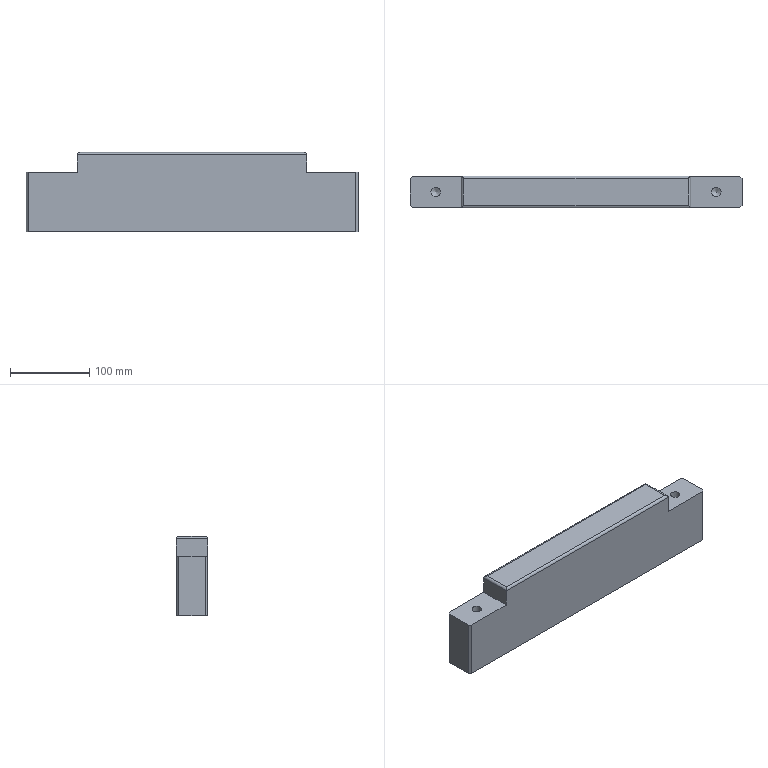Part | NX | features solid 2 | 1 solid | 26 faces | box 420 x 40 x 100 mm | volume 1534744 mm3 | plane 16 | cylinder 8 | cone 2 | commonest cylinder face diameters 6 x4 9 x2 12 x2
STEP:
#1=CARTESIAN_POINT('',(-323.,-106.5,359.));
#2=VERTEX_POINT('',#1);
#3=CARTESIAN_POINT('',(-323.,-106.5,363.5));
#4=DIRECTION('',(0.,-1.,0.));
#5=DIRECTION('',(0.,0.,-1.));
#6=AXIS2_PLACEMENT_3D('',#3,#4,#5);
#7=CIRCLE('',#6,4.5);
#8=EDGE_CURVE('',#2,#2,#7,.T.);
#9=ORIENTED_EDGE('',*,*,#8,.T.);
#10=EDGE_LOOP('',(#9));
#11=FACE_BOUND('',#10,.T.);
#12=CARTESIAN_POINT('',(-268.,-106.5,359.));
#13=VERTEX_POINT('',#12);
#14=CARTESIAN_POINT('',(-268.,-106.5,363.5));
#15=DIRECTION('',(0.,-1.,0.));
#16=DIRECTION('',(0.,0.,-1.));
#17=AXIS2_PLACEMENT_3D('',#14,#15,#16);
#18=CIRCLE('',#17,4.5);
#19=EDGE_CURVE('',#13,#13,#18,.T.);
#20=ORIENTED_EDGE('',*,*,#19,.T.);
#21=EDGE_LOOP('',(#20));
#22=FACE_BOUND('',#21,.T.);
#23=CARTESIAN_POINT('',(-150.,-106.5,402.));
#24=VERTEX_POINT('',#23);
#25=CARTESIAN_POINT('',(-440.,-106.5,402.));
#26=VERTEX_POINT('',#25);
#27=CARTESIAN_POINT('',(-440.,-106.5,402.));
#28=DIRECTION('',(-1.,0.,0.));
#29=VECTOR('',#28,1000.);
#30=LINE('',#27,#29);
#31=EDGE_CURVE('',#24,#26,#30,.T.);
#32=ORIENTED_EDGE('',*,*,#31,.F.);
#33=CARTESIAN_POINT('',(-150.,-106.5,380.));
#34=VERTEX_POINT('',#33);
#35=CARTESIAN_POINT('',(-150.,-106.5,380.));
#36=DIRECTION('',(0.,0.,1.));
#37=VECTOR('',#36,1000.);
#38=LINE('',#35,#37);
#39=EDGE_CURVE('',#34,#24,#38,.T.);
#40=ORIENTED_EDGE('',*,*,#39,.F.);
#41=CARTESIAN_POINT('',(-88.,-106.5,380.));
#42=VERTEX_POINT('',#41);
#43=CARTESIAN_POINT('',(-500.,-106.5,380.));
#44=DIRECTION('',(1.,0.,0.));
#45=VECTOR('',#44,1000.);
#46=LINE('',#43,#45);
#47=EDGE_CURVE('',#34,#42,#46,.T.);
#48=ORIENTED_EDGE('',*,*,#47,.T.);
#49=CARTESIAN_POINT('',(-88.,-106.5,305.));
#50=VERTEX_POINT('',#49);
#51=CARTESIAN_POINT('',(-88.,-106.5,380.));
#52=DIRECTION('',(0.,0.,1.));
#53=VECTOR('',#52,1000.);
#54=LINE('',#51,#53);
#55=EDGE_CURVE('',#50,#42,#54,.T.);
#56=ORIENTED_EDGE('',*,*,#55,.F.);
#57=CARTESIAN_POINT('',(-502.,-106.5,305.));
#58=VERTEX_POINT('',#57);
#59=CARTESIAN_POINT('',(-570.,-106.5,305.));
#60=DIRECTION('',(1.,0.,0.));
#61=VECTOR('',#60,1000.);
#62=LINE('',#59,#61);
#63=EDGE_CURVE('',#58,#50,#62,.T.);
#64=ORIENTED_EDGE('',*,*,#63,.F.);
#65=CARTESIAN_POINT('',(-502.,-106.5,380.));
#66=VERTEX_POINT('',#65);
#67=CARTESIAN_POINT('',(-502.,-106.5,380.));
#68=DIRECTION('',(0.,0.,-1.));
#69=VECTOR('',#68,1000.);
#70=LINE('',#67,#69);
#71=EDGE_CURVE('',#66,#58,#70,.T.);
#72=ORIENTED_EDGE('',*,*,#71,.F.);
#73=CARTESIAN_POINT('',(-440.,-106.5,380.));
#74=VERTEX_POINT('',#73);
#75=CARTESIAN_POINT('',(-570.,-106.5,380.));
#76=DIRECTION('',(1.,0.,0.));
#77=VECTOR('',#76,1000.);
#78=LINE('',#75,#77);
#79=EDGE_CURVE('',#66,#74,#78,.T.);
#80=ORIENTED_EDGE('',*,*,#79,.T.);
#81=CARTESIAN_POINT('',(-440.,-106.5,405.));
#82=DIRECTION('',(0.,0.,-1.));
#83=VECTOR('',#82,1000.);
#84=LINE('',#81,#83);
#85=EDGE_CURVE('',#74,#26,#84,.F.);
#86=ORIENTED_EDGE('',*,*,#85,.T.);
#87=EDGE_LOOP('',(#32,#40,#48,#56,#64,#72,#80,#86));
#88=FACE_BOUND('',#87,.T.);
#89=CARTESIAN_POINT('',(-570.,-106.5,380.));
#90=DIRECTION('',(0.,-1.,0.));
#91=DIRECTION('',(0.,0.,1.));
#92=AXIS2_PLACEMENT_3D('',#89,#90,#91);
#93=PLANE('',#92);
#94=ADVANCED_FACE('',(#11,#22,#88),#93,.F.);
#95=ORIENTED_EDGE('',*,*,#63,.T.);
#96=CARTESIAN_POINT('',(-85.,-109.5,305.));
#97=VERTEX_POINT('',#96);
#98=CARTESIAN_POINT('',(-85.,-109.5,305.));
#99=DIRECTION('',(0.7071,-0.7071,0.));
#100=VECTOR('',#99,1000.);
#101=LINE('',#98,#100);
#102=EDGE_CURVE('',#97,#50,#101,.F.);
#103=ORIENTED_EDGE('',*,*,#102,.F.);
#104=CARTESIAN_POINT('',(-85.,-143.5,305.));
#105=VERTEX_POINT('',#104);
#106=CARTESIAN_POINT('',(-85.,-106.5,305.));
#107=DIRECTION('',(0.,-1.,0.));
#108=VECTOR('',#107,1000.);
#109=LINE('',#106,#108);
#110=EDGE_CURVE('',#97,#105,#109,.T.);
#111=ORIENTED_EDGE('',*,*,#110,.T.);
#112=CARTESIAN_POINT('',(-88.,-146.5,305.));
#113=VERTEX_POINT('',#112);
#114=CARTESIAN_POINT('',(-88.,-146.5,305.));
#115=DIRECTION('',(-0.7071,-0.7071,0.));
#116=VECTOR('',#115,1000.);
#117=LINE('',#114,#116);
#118=EDGE_CURVE('',#113,#105,#117,.F.);
#119=ORIENTED_EDGE('',*,*,#118,.F.);
#120=CARTESIAN_POINT('',(-502.,-146.5,305.));
#121=VERTEX_POINT('',#120);
#122=CARTESIAN_POINT('',(-150.,-146.5,305.));
#123=DIRECTION('',(-1.,0.,0.));
#124=VECTOR('',#123,1000.);
#125=LINE('',#122,#124);
#126=EDGE_CURVE('',#113,#121,#125,.T.);
#127=ORIENTED_EDGE('',*,*,#126,.T.);
#128=CARTESIAN_POINT('',(-505.,-143.5,305.));
#129=VERTEX_POINT('',#128);
#130=CARTESIAN_POINT('',(-505.,-143.5,305.));
#131=DIRECTION('',(-0.7071,0.7071,0.));
#132=VECTOR('',#131,1000.);
#133=LINE('',#130,#132);
#134=EDGE_CURVE('',#129,#121,#133,.F.);
#135=ORIENTED_EDGE('',*,*,#134,.F.);
#136=CARTESIAN_POINT('',(-505.,-109.5,305.));
#137=VERTEX_POINT('',#136);
#138=CARTESIAN_POINT('',(-505.,-137.5,305.));
#139=DIRECTION('',(0.,1.,0.));
#140=VECTOR('',#139,1000.);
#141=LINE('',#138,#140);
#142=EDGE_CURVE('',#129,#137,#141,.T.);
#143=ORIENTED_EDGE('',*,*,#142,.T.);
#144=CARTESIAN_POINT('',(-502.,-106.5,305.));
#145=DIRECTION('',(0.7071,0.7071,0.));
#146=VECTOR('',#145,1000.);
#147=LINE('',#144,#146);
#148=EDGE_CURVE('',#58,#137,#147,.F.);
#149=ORIENTED_EDGE('',*,*,#148,.F.);
#150=EDGE_LOOP('',(#95,#103,#111,#119,#127,#135,#143,#149));
#151=FACE_BOUND('',#150,.T.);
#152=CARTESIAN_POINT('',(-470.,-127.5,305.));
#153=DIRECTION('',(0.,0.,1.));
#154=DIRECTION('',(1.,0.,0.));
#155=AXIS2_PLACEMENT_3D('',#152,#153,#154);
#156=PLANE('',#155);
#157=ADVANCED_FACE('',(#151),#156,.F.);
#158=ORIENTED_EDGE('',*,*,#126,.F.);
#159=CARTESIAN_POINT('',(-88.,-146.5,380.));
#160=VERTEX_POINT('',#159);
#161=CARTESIAN_POINT('',(-88.,-146.5,380.));
#162=DIRECTION('',(0.,0.,-1.));
#163=VECTOR('',#162,1000.);
#164=LINE('',#161,#163);
#165=EDGE_CURVE('',#160,#113,#164,.T.);
#166=ORIENTED_EDGE('',*,*,#165,.F.);
#167=CARTESIAN_POINT('',(-150.,-146.5,380.));
#168=VERTEX_POINT('',#167);
#169=CARTESIAN_POINT('',(-80.,-146.5,380.));
#170=DIRECTION('',(-1.,0.,0.));
#171=VECTOR('',#170,1000.);
#172=LINE('',#169,#171);
#173=EDGE_CURVE('',#160,#168,#172,.T.);
#174=ORIENTED_EDGE('',*,*,#173,.T.);
#175=CARTESIAN_POINT('',(-150.,-146.5,402.));
#176=VERTEX_POINT('',#175);
#177=CARTESIAN_POINT('',(-150.,-146.5,405.));
#178=DIRECTION('',(0.,0.,1.));
#179=VECTOR('',#178,1000.);
#180=LINE('',#177,#179);
#181=EDGE_CURVE('',#168,#176,#180,.T.);
#182=ORIENTED_EDGE('',*,*,#181,.T.);
#183=CARTESIAN_POINT('',(-440.,-146.5,402.));
#184=VERTEX_POINT('',#183);
#185=CARTESIAN_POINT('',(-220.,-146.5,402.));
#186=DIRECTION('',(1.,0.,0.));
#187=VECTOR('',#186,1000.);
#188=LINE('',#185,#187);
#189=EDGE_CURVE('',#184,#176,#188,.T.);
#190=ORIENTED_EDGE('',*,*,#189,.F.);
#191=CARTESIAN_POINT('',(-440.,-146.5,380.));
#192=VERTEX_POINT('',#191);
#193=CARTESIAN_POINT('',(-440.,-146.5,380.));
#194=DIRECTION('',(0.,0.,-1.));
#195=VECTOR('',#194,1000.);
#196=LINE('',#193,#195);
#197=EDGE_CURVE('',#192,#184,#196,.F.);
#198=ORIENTED_EDGE('',*,*,#197,.F.);
#199=CARTESIAN_POINT('',(-502.,-146.5,380.));
#200=VERTEX_POINT('',#199);
#201=CARTESIAN_POINT('',(-150.,-146.5,380.));
#202=DIRECTION('',(-1.,0.,0.));
#203=VECTOR('',#202,1000.);
#204=LINE('',#201,#203);
#205=EDGE_CURVE('',#192,#200,#204,.T.);
#206=ORIENTED_EDGE('',*,*,#205,.T.);
#207=CARTESIAN_POINT('',(-502.,-146.5,380.));
#208=DIRECTION('',(0.,0.,1.));
#209=VECTOR('',#208,1000.);
#210=LINE('',#207,#209);
#211=EDGE_CURVE('',#121,#200,#210,.T.);
#212=ORIENTED_EDGE('',*,*,#211,.F.);
#213=EDGE_LOOP('',(#158,#166,#174,#182,#190,#198,#206,#212));
#214=FACE_BOUND('',#213,.T.);
#215=CARTESIAN_POINT('',(-150.,-146.5,380.));
#216=DIRECTION('',(0.,1.,0.));
#217=DIRECTION('',(0.,0.,-1.));
#218=AXIS2_PLACEMENT_3D('',#215,#216,#217);
#219=PLANE('',#218);
#220=ADVANCED_FACE('',(#214),#219,.F.);
#221=CARTESIAN_POINT('',(-153.,-143.5,405.));
#222=VERTEX_POINT('',#221);
#223=CARTESIAN_POINT('',(-437.,-143.5,405.));
#224=VERTEX_POINT('',#223);
#225=CARTESIAN_POINT('',(-440.,-143.5,405.));
#226=DIRECTION('',(1.,0.,0.));
#227=VECTOR('',#226,1000.);
#228=LINE('',#225,#227);
#229=EDGE_CURVE('',#222,#224,#228,.F.);
#230=ORIENTED_EDGE('',*,*,#229,.F.);
#231=CARTESIAN_POINT('',(-153.,-109.5,405.));
#232=VERTEX_POINT('',#231);
#233=CARTESIAN_POINT('',(-153.,-146.5,405.));
#234=DIRECTION('',(0.,1.,0.));
#235=VECTOR('',#234,1000.);
#236=LINE('',#233,#235);
#237=EDGE_CURVE('',#232,#222,#236,.F.);
#238=ORIENTED_EDGE('',*,*,#237,.F.);
#239=CARTESIAN_POINT('',(-437.,-109.5,405.));
#240=VERTEX_POINT('',#239);
#241=CARTESIAN_POINT('',(-220.,-109.5,405.));
#242=DIRECTION('',(-1.,0.,0.));
#243=VECTOR('',#242,1000.);
#244=LINE('',#241,#243);
#245=EDGE_CURVE('',#240,#232,#244,.F.);
#246=ORIENTED_EDGE('',*,*,#245,.F.);
#247=CARTESIAN_POINT('',(-437.,-106.5,405.));
#248=DIRECTION('',(0.,1.,0.));
#249=VECTOR('',#248,1000.);
#250=LINE('',#247,#249);
#251=EDGE_CURVE('',#224,#240,#250,.T.);
#252=ORIENTED_EDGE('',*,*,#251,.F.);
#253=EDGE_LOOP('',(#230,#238,#246,#252));
#254=FACE_BOUND('',#253,.T.);
#255=CARTESIAN_POINT('',(-505.,89.,405.));
#256=DIRECTION('',(0.,0.,1.));
#257=DIRECTION('',(1.,0.,0.));
#258=AXIS2_PLACEMENT_3D('',#255,#256,#257);
#259=PLANE('',#258);
#260=ADVANCED_FACE('',(#254),#259,.T.);
#261=ORIENTED_EDGE('',*,*,#245,.T.);
#262=CARTESIAN_POINT('',(-153.,-109.5,402.));
#263=DIRECTION('',(-0.7071,0.7071,0.));
#264=DIRECTION('',(-0.7071,-0.7071,0.));
#265=AXIS2_PLACEMENT_3D('',#262,#263,#264);
#266=ELLIPSE('',#265,4.243,3.);
#267=EDGE_CURVE('',#24,#232,#266,.F.);
#268=ORIENTED_EDGE('',*,*,#267,.F.);
#269=ORIENTED_EDGE('',*,*,#31,.T.);
#270=CARTESIAN_POINT('',(-437.,-109.5,402.));
#271=DIRECTION('',(-0.7071,-0.7071,0.));
#272=DIRECTION('',(0.7071,-0.7071,0.));
#273=AXIS2_PLACEMENT_3D('',#270,#271,#272);
#274=ELLIPSE('',#273,4.243,3.);
#275=EDGE_CURVE('',#26,#240,#274,.F.);
#276=ORIENTED_EDGE('',*,*,#275,.T.);
#277=EDGE_LOOP('',(#261,#268,#269,#276));
#278=FACE_BOUND('',#277,.T.);
#279=CARTESIAN_POINT('',(-570.,-109.5,402.));
#280=DIRECTION('',(1.,0.,0.));
#281=DIRECTION('',(0.,0.,1.));
#282=AXIS2_PLACEMENT_3D('',#279,#280,#281);
#283=CYLINDRICAL_SURFACE('',#282,3.);
#284=ADVANCED_FACE('',(#278),#283,.T.);
#285=ORIENTED_EDGE('',*,*,#189,.T.);
#286=CARTESIAN_POINT('',(-153.,-143.5,402.));
#287=DIRECTION('',(0.7071,0.7071,0.));
#288=DIRECTION('',(0.7071,-0.7071,0.));
#289=AXIS2_PLACEMENT_3D('',#286,#287,#288);
#290=ELLIPSE('',#289,4.243,3.);
#291=EDGE_CURVE('',#222,#176,#290,.T.);
#292=ORIENTED_EDGE('',*,*,#291,.F.);
#293=ORIENTED_EDGE('',*,*,#229,.T.);
#294=CARTESIAN_POINT('',(-437.,-143.5,402.));
#295=DIRECTION('',(0.7071,-0.7071,0.));
#296=DIRECTION('',(-0.7071,-0.7071,0.));
#297=AXIS2_PLACEMENT_3D('',#294,#295,#296);
#298=ELLIPSE('',#297,4.243,3.);
#299=EDGE_CURVE('',#224,#184,#298,.T.);
#300=ORIENTED_EDGE('',*,*,#299,.T.);
#301=EDGE_LOOP('',(#285,#292,#293,#300));
#302=FACE_BOUND('',#301,.T.);
#303=CARTESIAN_POINT('',(-150.,-143.5,402.));
#304=DIRECTION('',(-1.,0.,0.));
#305=DIRECTION('',(0.,0.,-1.));
#306=AXIS2_PLACEMENT_3D('',#303,#304,#305);
#307=CYLINDRICAL_SURFACE('',#306,3.);
#308=ADVANCED_FACE('',(#302),#307,.T.);
#309=CARTESIAN_POINT('',(-466.5,-126.5,380.));
#310=VERTEX_POINT('',#309);
#311=CARTESIAN_POINT('',(-472.5,-126.5,380.));
#312=DIRECTION('',(0.,0.,1.));
#313=DIRECTION('',(1.,0.,0.));
#314=AXIS2_PLACEMENT_3D('',#311,#312,#313);
#315=CIRCLE('',#314,6.);
#316=EDGE_CURVE('',#310,#310,#315,.T.);
#317=ORIENTED_EDGE('',*,*,#316,.F.);
#318=EDGE_LOOP('',(#317));
#319=FACE_BOUND('',#318,.T.);
#320=ORIENTED_EDGE('',*,*,#205,.F.);
#321=CARTESIAN_POINT('',(-440.,-116.5,380.));
#322=DIRECTION('',(0.,1.,0.));
#323=VECTOR('',#322,1000.);
#324=LINE('',#321,#323);
#325=EDGE_CURVE('',#74,#192,#324,.F.);
#326=ORIENTED_EDGE('',*,*,#325,.F.);
#327=ORIENTED_EDGE('',*,*,#79,.F.);
#328=CARTESIAN_POINT('',(-505.,-109.5,380.));
#329=VERTEX_POINT('',#328);
#330=CARTESIAN_POINT('',(-496.5,-101.,380.));
#331=DIRECTION('',(-0.7071,-0.7071,0.));
#332=VECTOR('',#331,1000.);
#333=LINE('',#330,#332);
#334=EDGE_CURVE('',#329,#66,#333,.F.);
#335=ORIENTED_EDGE('',*,*,#334,.F.);
#336=CARTESIAN_POINT('',(-505.,-143.5,380.));
#337=VERTEX_POINT('',#336);
#338=CARTESIAN_POINT('',(-505.,-137.5,380.));
#339=DIRECTION('',(0.,1.,0.));
#340=VECTOR('',#339,1000.);
#341=LINE('',#338,#340);
#342=EDGE_CURVE('',#337,#329,#341,.T.);
#343=ORIENTED_EDGE('',*,*,#342,.F.);
#344=CARTESIAN_POINT('',(-495.5,-153.,380.));
#345=DIRECTION('',(0.7071,-0.7071,0.));
#346=VECTOR('',#345,1000.);
#347=LINE('',#344,#346);
#348=EDGE_CURVE('',#200,#337,#347,.F.);
#349=ORIENTED_EDGE('',*,*,#348,.F.);
#350=EDGE_LOOP('',(#320,#326,#327,#335,#343,#349));
#351=FACE_BOUND('',#350,.T.);
#352=CARTESIAN_POINT('',(-470.,-127.5,380.));
#353=DIRECTION('',(0.,0.,1.));
#354=DIRECTION('',(1.,0.,0.));
#355=AXIS2_PLACEMENT_3D('',#352,#353,#354);
#356=PLANE('',#355);
#357=ADVANCED_FACE('',(#319,#351),#356,.T.);
#358=ORIENTED_EDGE('',*,*,#342,.T.);
#359=CARTESIAN_POINT('',(-505.,-109.5,380.));
#360=DIRECTION('',(0.,0.,1.));
#361=VECTOR('',#360,1000.);
#362=LINE('',#359,#361);
#363=EDGE_CURVE('',#137,#329,#362,.T.);
#364=ORIENTED_EDGE('',*,*,#363,.F.);
#365=ORIENTED_EDGE('',*,*,#142,.F.);
#366=CARTESIAN_POINT('',(-505.,-143.5,380.));
#367=DIRECTION('',(0.,0.,-1.));
#368=VECTOR('',#367,1000.);
#369=LINE('',#366,#368);
#370=EDGE_CURVE('',#337,#129,#369,.T.);
#371=ORIENTED_EDGE('',*,*,#370,.F.);
#372=EDGE_LOOP('',(#358,#364,#365,#371));
#373=FACE_BOUND('',#372,.T.);
#374=CARTESIAN_POINT('',(-505.,-137.5,380.));
#375=DIRECTION('',(1.,0.,0.));
#376=DIRECTION('',(0.,0.,-1.));
#377=AXIS2_PLACEMENT_3D('',#374,#375,#376);
#378=PLANE('',#377);
#379=ADVANCED_FACE('',(#373),#378,.F.);
#380=ORIENTED_EDGE('',*,*,#85,.F.);
#381=ORIENTED_EDGE('',*,*,#325,.T.);
#382=ORIENTED_EDGE('',*,*,#197,.T.);
#383=CARTESIAN_POINT('',(-440.,-146.5,402.));
#384=DIRECTION('',(0.,-1.,0.));
#385=VECTOR('',#384,1000.);
#386=LINE('',#383,#385);
#387=EDGE_CURVE('',#26,#184,#386,.T.);
#388=ORIENTED_EDGE('',*,*,#387,.F.);
#389=EDGE_LOOP('',(#380,#381,#382,#388));
#390=FACE_BOUND('',#389,.T.);
#391=CARTESIAN_POINT('',(-440.,89.,405.));
#392=DIRECTION('',(-1.,0.,0.));
#393=DIRECTION('',(0.,0.,1.));
#394=AXIS2_PLACEMENT_3D('',#391,#392,#393);
#395=PLANE('',#394);
#396=ADVANCED_FACE('',(#390),#395,.T.);
#397=CARTESIAN_POINT('',(-466.5,-126.5,345.));
#398=VERTEX_POINT('',#397);
#399=CARTESIAN_POINT('',(-472.5,-126.5,345.));
#400=DIRECTION('',(0.,0.,1.));
#401=DIRECTION('',(1.,0.,0.));
#402=AXIS2_PLACEMENT_3D('',#399,#400,#401);
#403=CIRCLE('',#402,6.);
#404=EDGE_CURVE('',#398,#398,#403,.T.);
#405=ORIENTED_EDGE('',*,*,#404,.T.);
#406=EDGE_LOOP('',(#405));
#407=FACE_BOUND('',#406,.T.);
#408=CARTESIAN_POINT('',(-472.5,-126.5,341.395));
#409=VERTEX_POINT('',#408);
#410=VERTEX_LOOP('',#409);
#411=FACE_BOUND('',#410,.T.);
#412=CARTESIAN_POINT('',(-472.5,-126.5,345.));
#413=DIRECTION('',(0.,0.,1.));
#414=DIRECTION('',(-1.,0.,0.));
#415=AXIS2_PLACEMENT_3D('',#412,#413,#414);
#416=CONICAL_SURFACE('',#415,6.,1.03);
#417=ADVANCED_FACE('',(#407,#411),#416,.F.);
#418=ORIENTED_EDGE('',*,*,#404,.F.);
#419=EDGE_LOOP('',(#418));
#420=FACE_BOUND('',#419,.T.);
#421=ORIENTED_EDGE('',*,*,#316,.T.);
#422=EDGE_LOOP('',(#421));
#423=FACE_BOUND('',#422,.T.);
#424=CARTESIAN_POINT('',(-472.5,-126.5,380.));
#425=DIRECTION('',(0.,0.,-1.));
#426=DIRECTION('',(1.,0.,0.));
#427=AXIS2_PLACEMENT_3D('',#424,#425,#426);
#428=CYLINDRICAL_SURFACE('',#427,6.);
#429=ADVANCED_FACE('',(#420,#423),#428,.F.);
#430=ORIENTED_EDGE('',*,*,#348,.T.);
#431=ORIENTED_EDGE('',*,*,#370,.T.);
#432=ORIENTED_EDGE('',*,*,#134,.T.);
#433=ORIENTED_EDGE('',*,*,#211,.T.);
#434=EDGE_LOOP('',(#430,#431,#432,#433));
#435=FACE_BOUND('',#434,.T.);
#436=CARTESIAN_POINT('',(-505.,-143.5,380.));
#437=DIRECTION('',(0.7071,0.7071,0.));
#438=DIRECTION('',(0.7071,-0.7071,0.));
#439=AXIS2_PLACEMENT_3D('',#436,#437,#438);
#440=PLANE('',#439);
#441=ADVANCED_FACE('',(#435),#440,.F.);
#442=ORIENTED_EDGE('',*,*,#334,.T.);
#443=ORIENTED_EDGE('',*,*,#71,.T.);
#444=ORIENTED_EDGE('',*,*,#148,.T.);
#445=ORIENTED_EDGE('',*,*,#363,.T.);
#446=EDGE_LOOP('',(#442,#443,#444,#445));
#447=FACE_BOUND('',#446,.T.);
#448=CARTESIAN_POINT('',(-502.,-106.5,380.));
#449=DIRECTION('',(0.7071,-0.7071,0.));
#450=DIRECTION('',(-0.7071,-0.7071,0.));
#451=AXIS2_PLACEMENT_3D('',#448,#449,#450);
#452=PLANE('',#451);
#453=ADVANCED_FACE('',(#447),#452,.F.);
#454=ORIENTED_EDGE('',*,*,#275,.F.);
#455=ORIENTED_EDGE('',*,*,#387,.T.);
#456=ORIENTED_EDGE('',*,*,#299,.F.);
#457=ORIENTED_EDGE('',*,*,#251,.T.);
#458=EDGE_LOOP('',(#454,#455,#456,#457));
#459=FACE_BOUND('',#458,.T.);
#460=CARTESIAN_POINT('',(-437.,89.,402.));
#461=DIRECTION('',(0.,-1.,0.));
#462=DIRECTION('',(0.,0.,-1.));
#463=AXIS2_PLACEMENT_3D('',#460,#461,#462);
#464=CYLINDRICAL_SURFACE('',#463,3.);
#465=ADVANCED_FACE('',(#459),#464,.T.);
#466=CARTESIAN_POINT('',(-111.5,-126.5,345.));
#467=VERTEX_POINT('',#466);
#468=CARTESIAN_POINT('',(-117.5,-126.5,345.));
#469=DIRECTION('',(0.,0.,1.));
#470=DIRECTION('',(1.,0.,0.));
#471=AXIS2_PLACEMENT_3D('',#468,#469,#470);
#472=CIRCLE('',#471,6.);
#473=EDGE_CURVE('',#467,#467,#472,.T.);
#474=ORIENTED_EDGE('',*,*,#473,.T.);
#475=EDGE_LOOP('',(#474));
#476=FACE_BOUND('',#475,.T.);
#477=CARTESIAN_POINT('',(-117.5,-126.5,341.395));
#478=VERTEX_POINT('',#477);
#479=VERTEX_LOOP('',#478);
#480=FACE_BOUND('',#479,.T.);
#481=CARTESIAN_POINT('',(-117.5,-126.5,345.));
#482=DIRECTION('',(0.,0.,1.));
#483=DIRECTION('',(-1.,0.,0.));
#484=AXIS2_PLACEMENT_3D('',#481,#482,#483);
#485=CONICAL_SURFACE('',#484,6.,1.03);
#486=ADVANCED_FACE('',(#476,#480),#485,.F.);
#487=ORIENTED_EDGE('',*,*,#473,.F.);
#488=EDGE_LOOP('',(#487));
#489=FACE_BOUND('',#488,.T.);
#490=CARTESIAN_POINT('',(-111.5,-126.5,380.));
#491=VERTEX_POINT('',#490);
#492=CARTESIAN_POINT('',(-117.5,-126.5,380.));
#493=DIRECTION('',(0.,0.,1.));
#494=DIRECTION('',(1.,0.,0.));
#495=AXIS2_PLACEMENT_3D('',#492,#493,#494);
#496=CIRCLE('',#495,6.);
#497=EDGE_CURVE('',#491,#491,#496,.T.);
#498=ORIENTED_EDGE('',*,*,#497,.T.);
#499=EDGE_LOOP('',(#498));
#500=FACE_BOUND('',#499,.T.);
#501=CARTESIAN_POINT('',(-117.5,-126.5,380.));
#502=DIRECTION('',(0.,0.,-1.));
#503=DIRECTION('',(1.,0.,0.));
#504=AXIS2_PLACEMENT_3D('',#501,#502,#503);
#505=CYLINDRICAL_SURFACE('',#504,6.);
#506=ADVANCED_FACE('',(#489,#500),#505,.F.);
#507=CARTESIAN_POINT('',(-85.,-109.5,380.));
#508=VERTEX_POINT('',#507);
#509=CARTESIAN_POINT('',(-85.,-143.5,380.));
#510=VERTEX_POINT('',#509);
#511=CARTESIAN_POINT('',(-85.,-106.5,380.));
#512=DIRECTION('',(0.,-1.,0.));
#513=VECTOR('',#512,1000.);
#514=LINE('',#511,#513);
#515=EDGE_CURVE('',#508,#510,#514,.T.);
#516=ORIENTED_EDGE('',*,*,#515,.T.);
#517=CARTESIAN_POINT('',(-85.,-143.5,380.));
#518=DIRECTION('',(0.,0.,1.));
#519=VECTOR('',#518,1000.);
#520=LINE('',#517,#519);
#521=EDGE_CURVE('',#105,#510,#520,.T.);
#522=ORIENTED_EDGE('',*,*,#521,.F.);
#523=ORIENTED_EDGE('',*,*,#110,.F.);
#524=CARTESIAN_POINT('',(-85.,-109.5,380.));
#525=DIRECTION('',(0.,0.,-1.));
#526=VECTOR('',#525,1000.);
#527=LINE('',#524,#526);
#528=EDGE_CURVE('',#508,#97,#527,.T.);
#529=ORIENTED_EDGE('',*,*,#528,.F.);
#530=EDGE_LOOP('',(#516,#522,#523,#529));
#531=FACE_BOUND('',#530,.T.);
#532=CARTESIAN_POINT('',(-85.,-106.5,380.));
#533=DIRECTION('',(-1.,0.,0.));
#534=DIRECTION('',(0.,0.,1.));
#535=AXIS2_PLACEMENT_3D('',#532,#533,#534);
#536=PLANE('',#535);
#537=ADVANCED_FACE('',(#531),#536,.F.);
#538=CARTESIAN_POINT('',(-85.,-109.5,380.));
#539=DIRECTION('',(0.7071,-0.7071,0.));
#540=VECTOR('',#539,1000.);
#541=LINE('',#538,#540);
#542=EDGE_CURVE('',#42,#508,#541,.T.);
#543=ORIENTED_EDGE('',*,*,#542,.T.);
#544=ORIENTED_EDGE('',*,*,#528,.T.);
#545=ORIENTED_EDGE('',*,*,#102,.T.);
#546=ORIENTED_EDGE('',*,*,#55,.T.);
#547=EDGE_LOOP('',(#543,#544,#545,#546));
#548=FACE_BOUND('',#547,.T.);
#549=CARTESIAN_POINT('',(-85.,-109.5,380.));
#550=DIRECTION('',(-0.7071,-0.7071,0.));
#551=DIRECTION('',(-0.7071,0.7071,0.));
#552=AXIS2_PLACEMENT_3D('',#549,#550,#551);
#553=PLANE('',#552);
#554=ADVANCED_FACE('',(#548),#553,.F.);
#555=ORIENTED_EDGE('',*,*,#181,.F.);
#556=CARTESIAN_POINT('',(-150.,-116.5,380.));
#557=DIRECTION('',(0.,1.,0.));
#558=VECTOR('',#557,1000.);
#559=LINE('',#556,#558);
#560=EDGE_CURVE('',#168,#34,#559,.T.);
#561=ORIENTED_EDGE('',*,*,#560,.T.);
#562=ORIENTED_EDGE('',*,*,#39,.T.);
#563=CARTESIAN_POINT('',(-150.,-106.5,402.));
#564=DIRECTION('',(0.,1.,0.));
#565=VECTOR('',#564,1000.);
#566=LINE('',#563,#565);
#567=EDGE_CURVE('',#176,#24,#566,.T.);
#568=ORIENTED_EDGE('',*,*,#567,.F.);
#569=EDGE_LOOP('',(#555,#561,#562,#568));
#570=FACE_BOUND('',#569,.T.);
#571=CARTESIAN_POINT('',(-150.,89.,405.));
#572=DIRECTION('',(-1.,0.,0.));
#573=DIRECTION('',(0.,0.,1.));
#574=AXIS2_PLACEMENT_3D('',#571,#572,#573);
#575=PLANE('',#574);
#576=ADVANCED_FACE('',(#570),#575,.F.);
#577=ORIENTED_EDGE('',*,*,#497,.F.);
#578=EDGE_LOOP('',(#577));
#579=FACE_BOUND('',#578,.T.);
#580=ORIENTED_EDGE('',*,*,#47,.F.);
#581=ORIENTED_EDGE('',*,*,#560,.F.);
#582=ORIENTED_EDGE('',*,*,#173,.F.);
#583=CARTESIAN_POINT('',(-88.,-146.5,380.));
#584=DIRECTION('',(-0.7071,-0.7071,0.));
#585=VECTOR('',#584,1000.);
#586=LINE('',#583,#585);
#587=EDGE_CURVE('',#510,#160,#586,.T.);
#588=ORIENTED_EDGE('',*,*,#587,.F.);
#589=ORIENTED_EDGE('',*,*,#515,.F.);
#590=ORIENTED_EDGE('',*,*,#542,.F.);
#591=EDGE_LOOP('',(#580,#581,#582,#588,#589,#590));
#592=FACE_BOUND('',#591,.T.);
#593=CARTESIAN_POINT('',(-400.,-127.5,380.));
#594=DIRECTION('',(0.,0.,1.));
#595=DIRECTION('',(1.,0.,0.));
#596=AXIS2_PLACEMENT_3D('',#593,#594,#595);
#597=PLANE('',#596);
#598=ADVANCED_FACE('',(#579,#592),#597,.T.);
#599=ORIENTED_EDGE('',*,*,#587,.T.);
#600=ORIENTED_EDGE('',*,*,#165,.T.);
#601=ORIENTED_EDGE('',*,*,#118,.T.);
#602=ORIENTED_EDGE('',*,*,#521,.T.);
#603=EDGE_LOOP('',(#599,#600,#601,#602));
#604=FACE_BOUND('',#603,.T.);
#605=CARTESIAN_POINT('',(-88.,-146.5,380.));
#606=DIRECTION('',(-0.7071,0.7071,0.));
#607=DIRECTION('',(0.7071,0.7071,0.));
#608=AXIS2_PLACEMENT_3D('',#605,#606,#607);
#609=PLANE('',#608);
#610=ADVANCED_FACE('',(#604),#609,.F.);
#611=ORIENTED_EDGE('',*,*,#291,.T.);
#612=ORIENTED_EDGE('',*,*,#567,.T.);
#613=ORIENTED_EDGE('',*,*,#267,.T.);
#614=ORIENTED_EDGE('',*,*,#237,.T.);
#615=EDGE_LOOP('',(#611,#612,#613,#614));
#616=FACE_BOUND('',#615,.T.);
#617=CARTESIAN_POINT('',(-153.,89.,402.));
#618=DIRECTION('',(0.,-1.,0.));
#619=DIRECTION('',(0.,0.,-1.));
#620=AXIS2_PLACEMENT_3D('',#617,#618,#619);
#621=CYLINDRICAL_SURFACE('',#620,3.);
#622=ADVANCED_FACE('',(#616),#621,.T.);
#623=CARTESIAN_POINT('',(-268.,-141.5,359.));
#624=VERTEX_POINT('',#623);
#625=CARTESIAN_POINT('',(-268.,-141.5,363.5));
#626=DIRECTION('',(0.000000011,-1.,0.00000017));
#627=DIRECTION('',(0.,-0.00000017,-1.));
#628=AXIS2_PLACEMENT_3D('',#625,#626,#627);
#629=CIRCLE('',#628,4.5);
#630=EDGE_CURVE('',#624,#624,#629,.T.);
#631=ORIENTED_EDGE('',*,*,#630,.T.);
#632=EDGE_LOOP('',(#631));
#633=FACE_BOUND('',#632,.T.);
#634=ORIENTED_EDGE('',*,*,#19,.F.);
#635=EDGE_LOOP('',(#634));
#636=FACE_BOUND('',#635,.T.);
#637=CARTESIAN_POINT('',(-268.,-81.5,363.5));
#638=DIRECTION('',(0.000000011,-1.,0.00000017));
#639=DIRECTION('',(0.,-0.00000017,-1.));
#640=AXIS2_PLACEMENT_3D('',#637,#638,#639);
#641=CYLINDRICAL_SURFACE('',#640,4.5);
#642=ADVANCED_FACE('',(#633,#636),#641,.F.);
#643=ORIENTED_EDGE('',*,*,#630,.F.);
#644=EDGE_LOOP('',(#643));
#645=FACE_BOUND('',#644,.T.);
#646=CARTESIAN_POINT('',(-268.,-141.5,363.5));
#647=DIRECTION('',(0.000000011,-1.,0.00000017));
#648=DIRECTION('',(0.,-0.00000017,-1.));
#649=AXIS2_PLACEMENT_3D('',#646,#647,#648);
#650=PLANE('',#649);
#651=ADVANCED_FACE('',(#645),#650,.F.);
#652=CARTESIAN_POINT('',(-323.,-141.5,359.));
#653=VERTEX_POINT('',#652);
#654=CARTESIAN_POINT('',(-323.,-141.5,363.5));
#655=DIRECTION('',(0.000000011,-1.,0.00000017));
#656=DIRECTION('',(0.,-0.00000017,-1.));
#657=AXIS2_PLACEMENT_3D('',#654,#655,#656);
#658=CIRCLE('',#657,4.5);
#659=EDGE_CURVE('',#653,#653,#658,.T.);
#660=ORIENTED_EDGE('',*,*,#659,.T.);
#661=EDGE_LOOP('',(#660));
#662=FACE_BOUND('',#661,.T.);
#663=ORIENTED_EDGE('',*,*,#8,.F.);
#664=EDGE_LOOP('',(#663));
#665=FACE_BOUND('',#664,.T.);
#666=CARTESIAN_POINT('',(-323.,-81.5,363.5));
#667=DIRECTION('',(0.000000011,-1.,0.00000017));
#668=DIRECTION('',(0.,-0.00000017,-1.));
#669=AXIS2_PLACEMENT_3D('',#666,#667,#668);
#670=CYLINDRICAL_SURFACE('',#669,4.5);
#671=ADVANCED_FACE('',(#662,#665),#670,.F.);
#672=ORIENTED_EDGE('',*,*,#659,.F.);
#673=EDGE_LOOP('',(#672));
#674=FACE_BOUND('',#673,.T.);
#675=CARTESIAN_POINT('',(-323.,-141.5,363.5));
#676=DIRECTION('',(0.000000011,-1.,0.00000017));
#677=DIRECTION('',(0.,-0.00000017,-1.));
#678=AXIS2_PLACEMENT_3D('',#675,#676,#677);
#679=PLANE('',#678);
#680=ADVANCED_FACE('',(#674),#679,.F.);
#681=CLOSED_SHELL('',(#94,#157,#220,#260,#284,#308,#357,#379,#396,#417,#429,#441,#453,#465,#486,#506,#537,#554,#576,#598,#610,#622,#642,#651,#671,#680));
#682=MANIFOLD_SOLID_BREP('',#681);
#683=(LENGTH_UNIT()NAMED_UNIT(*)SI_UNIT(.MILLI.,.METRE.));
#684=UNCERTAINTY_MEASURE_WITH_UNIT(LENGTH_MEASURE(0.00001),#683,'','');
#685=(NAMED_UNIT(*)PLANE_ANGLE_UNIT()SI_UNIT($,.RADIAN.));
#686=(NAMED_UNIT(*)SI_UNIT($,.STERADIAN.)SOLID_ANGLE_UNIT());
#687=(GEOMETRIC_REPRESENTATION_CONTEXT(3)GLOBAL_UNCERTAINTY_ASSIGNED_CONTEXT((#684))GLOBAL_UNIT_ASSIGNED_CONTEXT((#683,#685,#686))REPRESENTATION_CONTEXT('',''));
#688=ADVANCED_BREP_SHAPE_REPRESENTATION('',(#682),#687);